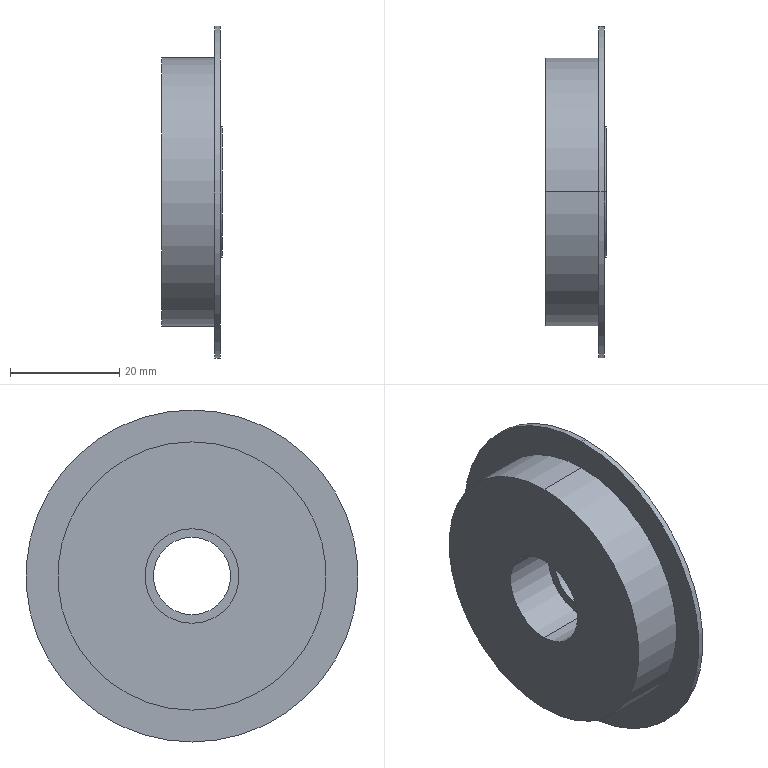Part | SolidWorks | features Revolution 1 | 2 solids | 18 faces | box 11.085 x 60.752 x 60.752 mm | volume 17812 mm3 | cylinder 12 | plane 6 | commonest cylinder face diameters 14.183 x2 17.319 x2 23.998 x2 45.246 x2 49.1 x2 60.752 x2
STEP:
#1=CARTESIAN_POINT('',(108.,0.,22.623));
#2=VERTEX_POINT('',#1);
#3=CARTESIAN_POINT('',(108.,0.,-22.623));
#4=VERTEX_POINT('',#3);
#5=CARTESIAN_POINT('',(108.,0.,0.));
#6=DIRECTION('',(1.,0.,0.));
#7=DIRECTION('',(0.,0.,-1.));
#8=AXIS2_PLACEMENT_3D('',#5,#6,#7);
#9=CIRCLE('',#8,22.623);
#10=EDGE_CURVE('',#2,#4,#9,.T.);
#11=ORIENTED_EDGE('',*,*,#10,.F.);
#12=CARTESIAN_POINT('',(109.025,0.,22.623));
#13=VERTEX_POINT('',#12);
#14=CARTESIAN_POINT('',(0.,0.,22.623));
#15=DIRECTION('',(1.,0.,0.));
#16=VECTOR('',#15,1000.);
#17=LINE('',#14,#16);
#18=EDGE_CURVE('',#2,#13,#17,.T.);
#19=ORIENTED_EDGE('',*,*,#18,.T.);
#20=CARTESIAN_POINT('',(109.025,0.,-22.623));
#21=VERTEX_POINT('',#20);
#22=CARTESIAN_POINT('',(109.025,0.,0.));
#23=DIRECTION('',(1.,0.,0.));
#24=DIRECTION('',(0.,0.,-1.));
#25=AXIS2_PLACEMENT_3D('',#22,#23,#24);
#26=CIRCLE('',#25,22.623);
#27=EDGE_CURVE('',#13,#21,#26,.T.);
#28=ORIENTED_EDGE('',*,*,#27,.T.);
#29=CARTESIAN_POINT('',(0.,0.,-22.623));
#30=DIRECTION('',(1.,0.,0.));
#31=VECTOR('',#30,1000.);
#32=LINE('',#29,#31);
#33=EDGE_CURVE('',#4,#21,#32,.T.);
#34=ORIENTED_EDGE('',*,*,#33,.F.);
#35=EDGE_LOOP('',(#11,#19,#28,#34));
#36=FACE_OUTER_BOUND('',#35,.T.);
#37=CARTESIAN_POINT('',(0.,0.,0.));
#38=DIRECTION('',(1.,0.,0.));
#39=DIRECTION('',(0.,0.,-1.));
#40=AXIS2_PLACEMENT_3D('',#37,#38,#39);
#41=CYLINDRICAL_SURFACE('',#40,22.623);
#42=ADVANCED_FACE('',(#36),#41,.F.);
#43=CARTESIAN_POINT('',(98.286,0.,8.66));
#44=VERTEX_POINT('',#43);
#45=CARTESIAN_POINT('',(98.286,0.,-8.66));
#46=VERTEX_POINT('',#45);
#47=CARTESIAN_POINT('',(98.286,0.,0.));
#48=DIRECTION('',(1.,0.,0.));
#49=DIRECTION('',(0.,0.,-1.));
#50=AXIS2_PLACEMENT_3D('',#47,#48,#49);
#51=CIRCLE('',#50,8.66);
#52=EDGE_CURVE('',#44,#46,#51,.T.);
#53=ORIENTED_EDGE('',*,*,#52,.F.);
#54=CARTESIAN_POINT('',(108.,0.,8.66));
#55=VERTEX_POINT('',#54);
#56=CARTESIAN_POINT('',(0.,0.,8.66));
#57=DIRECTION('',(1.,0.,0.));
#58=VECTOR('',#57,1000.);
#59=LINE('',#56,#58);
#60=EDGE_CURVE('',#44,#55,#59,.T.);
#61=ORIENTED_EDGE('',*,*,#60,.T.);
#62=CARTESIAN_POINT('',(108.,0.,-8.66));
#63=VERTEX_POINT('',#62);
#64=CARTESIAN_POINT('',(108.,0.,0.));
#65=DIRECTION('',(1.,0.,0.));
#66=DIRECTION('',(0.,0.,-1.));
#67=AXIS2_PLACEMENT_3D('',#64,#65,#66);
#68=CIRCLE('',#67,8.66);
#69=EDGE_CURVE('',#55,#63,#68,.T.);
#70=ORIENTED_EDGE('',*,*,#69,.T.);
#71=CARTESIAN_POINT('',(0.,0.,-8.66));
#72=DIRECTION('',(1.,0.,0.));
#73=VECTOR('',#72,1000.);
#74=LINE('',#71,#73);
#75=EDGE_CURVE('',#46,#63,#74,.T.);
#76=ORIENTED_EDGE('',*,*,#75,.F.);
#77=EDGE_LOOP('',(#53,#61,#70,#76));
#78=FACE_OUTER_BOUND('',#77,.T.);
#79=CARTESIAN_POINT('',(0.,0.,0.));
#80=DIRECTION('',(1.,0.,0.));
#81=DIRECTION('',(0.,0.,-1.));
#82=AXIS2_PLACEMENT_3D('',#79,#80,#81);
#83=CYLINDRICAL_SURFACE('',#82,8.66);
#84=ADVANCED_FACE('',(#78),#83,.F.);
#85=CARTESIAN_POINT('',(98.286,0.,-24.55));
#86=VERTEX_POINT('',#85);
#87=CARTESIAN_POINT('',(98.286,0.,24.55));
#88=VERTEX_POINT('',#87);
#89=CARTESIAN_POINT('',(98.286,0.,0.));
#90=DIRECTION('',(1.,0.,0.));
#91=DIRECTION('',(0.,0.,-1.));
#92=AXIS2_PLACEMENT_3D('',#89,#90,#91);
#93=CIRCLE('',#92,24.55);
#94=EDGE_CURVE('',#86,#88,#93,.T.);
#95=ORIENTED_EDGE('',*,*,#94,.T.);
#96=CARTESIAN_POINT('',(108.,0.,24.55));
#97=VERTEX_POINT('',#96);
#98=CARTESIAN_POINT('',(0.,0.,24.55));
#99=DIRECTION('',(1.,0.,0.));
#100=VECTOR('',#99,1000.);
#101=LINE('',#98,#100);
#102=EDGE_CURVE('',#88,#97,#101,.T.);
#103=ORIENTED_EDGE('',*,*,#102,.T.);
#104=CARTESIAN_POINT('',(108.,0.,-24.55));
#105=VERTEX_POINT('',#104);
#106=CARTESIAN_POINT('',(108.,0.,0.));
#107=DIRECTION('',(1.,0.,0.));
#108=DIRECTION('',(0.,0.,-1.));
#109=AXIS2_PLACEMENT_3D('',#106,#107,#108);
#110=CIRCLE('',#109,24.55);
#111=EDGE_CURVE('',#105,#97,#110,.T.);
#112=ORIENTED_EDGE('',*,*,#111,.F.);
#113=CARTESIAN_POINT('',(0.,0.,-24.55));
#114=DIRECTION('',(1.,0.,0.));
#115=VECTOR('',#114,1000.);
#116=LINE('',#113,#115);
#117=EDGE_CURVE('',#86,#105,#116,.T.);
#118=ORIENTED_EDGE('',*,*,#117,.F.);
#119=EDGE_LOOP('',(#95,#103,#112,#118));
#120=FACE_OUTER_BOUND('',#119,.T.);
#121=CARTESIAN_POINT('',(0.,0.,0.));
#122=DIRECTION('',(1.,0.,0.));
#123=DIRECTION('',(0.,0.,-1.));
#124=AXIS2_PLACEMENT_3D('',#121,#122,#123);
#125=CYLINDRICAL_SURFACE('',#124,24.55);
#126=ADVANCED_FACE('',(#120),#125,.T.);
#127=CARTESIAN_POINT('',(108.,0.,-30.376));
#128=VERTEX_POINT('',#127);
#129=CARTESIAN_POINT('',(108.,0.,30.376));
#130=VERTEX_POINT('',#129);
#131=CARTESIAN_POINT('',(108.,0.,0.));
#132=DIRECTION('',(1.,0.,0.));
#133=DIRECTION('',(0.,0.,-1.));
#134=AXIS2_PLACEMENT_3D('',#131,#132,#133);
#135=CIRCLE('',#134,30.376);
#136=EDGE_CURVE('',#128,#130,#135,.T.);
#137=ORIENTED_EDGE('',*,*,#136,.T.);
#138=CARTESIAN_POINT('',(109.025,0.,30.376));
#139=VERTEX_POINT('',#138);
#140=CARTESIAN_POINT('',(0.,0.,30.376));
#141=DIRECTION('',(1.,0.,0.));
#142=VECTOR('',#141,1000.);
#143=LINE('',#140,#142);
#144=EDGE_CURVE('',#130,#139,#143,.T.);
#145=ORIENTED_EDGE('',*,*,#144,.T.);
#146=CARTESIAN_POINT('',(109.025,0.,-30.376));
#147=VERTEX_POINT('',#146);
#148=CARTESIAN_POINT('',(109.025,0.,0.));
#149=DIRECTION('',(1.,0.,0.));
#150=DIRECTION('',(0.,0.,-1.));
#151=AXIS2_PLACEMENT_3D('',#148,#149,#150);
#152=CIRCLE('',#151,30.376);
#153=EDGE_CURVE('',#147,#139,#152,.T.);
#154=ORIENTED_EDGE('',*,*,#153,.F.);
#155=CARTESIAN_POINT('',(0.,0.,-30.376));
#156=DIRECTION('',(1.,0.,0.));
#157=VECTOR('',#156,1000.);
#158=LINE('',#155,#157);
#159=EDGE_CURVE('',#128,#147,#158,.T.);
#160=ORIENTED_EDGE('',*,*,#159,.F.);
#161=EDGE_LOOP('',(#137,#145,#154,#160));
#162=FACE_OUTER_BOUND('',#161,.T.);
#163=CARTESIAN_POINT('',(0.,0.,0.));
#164=DIRECTION('',(1.,0.,0.));
#165=DIRECTION('',(0.,0.,-1.));
#166=AXIS2_PLACEMENT_3D('',#163,#164,#165);
#167=CYLINDRICAL_SURFACE('',#166,30.376);
#168=ADVANCED_FACE('',(#162),#167,.T.);
#169=ORIENTED_EDGE('',*,*,#144,.F.);
#170=CARTESIAN_POINT('',(108.,0.,0.));
#171=DIRECTION('',(1.,0.,0.));
#172=DIRECTION('',(0.,0.,-1.));
#173=AXIS2_PLACEMENT_3D('',#170,#171,#172);
#174=CIRCLE('',#173,30.376);
#175=EDGE_CURVE('',#130,#128,#174,.T.);
#176=ORIENTED_EDGE('',*,*,#175,.T.);
#177=ORIENTED_EDGE('',*,*,#159,.T.);
#178=CARTESIAN_POINT('',(109.025,0.,0.));
#179=DIRECTION('',(1.,0.,0.));
#180=DIRECTION('',(0.,0.,-1.));
#181=AXIS2_PLACEMENT_3D('',#178,#179,#180);
#182=CIRCLE('',#181,30.376);
#183=EDGE_CURVE('',#139,#147,#182,.T.);
#184=ORIENTED_EDGE('',*,*,#183,.F.);
#185=EDGE_LOOP('',(#169,#176,#177,#184));
#186=FACE_OUTER_BOUND('',#185,.T.);
#187=CARTESIAN_POINT('',(0.,0.,0.));
#188=DIRECTION('',(1.,0.,0.));
#189=DIRECTION('',(0.,0.,-1.));
#190=AXIS2_PLACEMENT_3D('',#187,#188,#189);
#191=CYLINDRICAL_SURFACE('',#190,30.376);
#192=ADVANCED_FACE('',(#186),#191,.T.);
#193=ORIENTED_EDGE('',*,*,#111,.T.);
#194=CARTESIAN_POINT('',(108.,0.,0.));
#195=DIRECTION('',(1.,0.,0.));
#196=DIRECTION('',(0.,0.,-1.));
#197=AXIS2_PLACEMENT_3D('',#194,#195,#196);
#198=CIRCLE('',#197,24.55);
#199=EDGE_CURVE('',#97,#105,#198,.T.);
#200=ORIENTED_EDGE('',*,*,#199,.T.);
#201=EDGE_LOOP('',(#193,#200));
#202=FACE_BOUND('',#201,.T.);
#203=ORIENTED_EDGE('',*,*,#136,.F.);
#204=ORIENTED_EDGE('',*,*,#175,.F.);
#205=EDGE_LOOP('',(#203,#204));
#206=FACE_OUTER_BOUND('',#205,.T.);
#207=CARTESIAN_POINT('',(108.,30.376,0.));
#208=DIRECTION('',(-1.,0.,0.));
#209=DIRECTION('',(0.,0.,1.));
#210=AXIS2_PLACEMENT_3D('',#207,#208,#209);
#211=PLANE('',#210);
#212=ADVANCED_FACE('',(#202,#206),#211,.T.);
#213=ORIENTED_EDGE('',*,*,#102,.F.);
#214=CARTESIAN_POINT('',(98.286,0.,0.));
#215=DIRECTION('',(1.,0.,0.));
#216=DIRECTION('',(0.,0.,-1.));
#217=AXIS2_PLACEMENT_3D('',#214,#215,#216);
#218=CIRCLE('',#217,24.55);
#219=EDGE_CURVE('',#88,#86,#218,.T.);
#220=ORIENTED_EDGE('',*,*,#219,.T.);
#221=ORIENTED_EDGE('',*,*,#117,.T.);
#222=ORIENTED_EDGE('',*,*,#199,.F.);
#223=EDGE_LOOP('',(#213,#220,#221,#222));
#224=FACE_OUTER_BOUND('',#223,.T.);
#225=CARTESIAN_POINT('',(0.,0.,0.));
#226=DIRECTION('',(1.,0.,0.));
#227=DIRECTION('',(0.,0.,-1.));
#228=AXIS2_PLACEMENT_3D('',#225,#226,#227);
#229=CYLINDRICAL_SURFACE('',#228,24.55);
#230=ADVANCED_FACE('',(#224),#229,.T.);
#231=CARTESIAN_POINT('',(98.286,0.,0.));
#232=DIRECTION('',(1.,0.,0.));
#233=DIRECTION('',(0.,0.,-1.));
#234=AXIS2_PLACEMENT_3D('',#231,#232,#233);
#235=CIRCLE('',#234,8.66);
#236=EDGE_CURVE('',#46,#44,#235,.T.);
#237=ORIENTED_EDGE('',*,*,#236,.T.);
#238=ORIENTED_EDGE('',*,*,#52,.T.);
#239=EDGE_LOOP('',(#237,#238));
#240=FACE_BOUND('',#239,.T.);
#241=ORIENTED_EDGE('',*,*,#94,.F.);
#242=ORIENTED_EDGE('',*,*,#219,.F.);
#243=EDGE_LOOP('',(#241,#242));
#244=FACE_OUTER_BOUND('',#243,.T.);
#245=CARTESIAN_POINT('',(98.286,24.55,0.));
#246=DIRECTION('',(-1.,0.,0.));
#247=DIRECTION('',(0.,0.,1.));
#248=AXIS2_PLACEMENT_3D('',#245,#246,#247);
#249=PLANE('',#248);
#250=ADVANCED_FACE('',(#240,#244),#249,.T.);
#251=ORIENTED_EDGE('',*,*,#60,.F.);
#252=ORIENTED_EDGE('',*,*,#236,.F.);
#253=ORIENTED_EDGE('',*,*,#75,.T.);
#254=CARTESIAN_POINT('',(108.,0.,0.));
#255=DIRECTION('',(1.,0.,0.));
#256=DIRECTION('',(0.,0.,-1.));
#257=AXIS2_PLACEMENT_3D('',#254,#255,#256);
#258=CIRCLE('',#257,8.66);
#259=EDGE_CURVE('',#63,#55,#258,.T.);
#260=ORIENTED_EDGE('',*,*,#259,.T.);
#261=EDGE_LOOP('',(#251,#252,#253,#260));
#262=FACE_OUTER_BOUND('',#261,.T.);
#263=CARTESIAN_POINT('',(0.,0.,0.));
#264=DIRECTION('',(1.,0.,0.));
#265=DIRECTION('',(0.,0.,-1.));
#266=AXIS2_PLACEMENT_3D('',#263,#264,#265);
#267=CYLINDRICAL_SURFACE('',#266,8.66);
#268=ADVANCED_FACE('',(#262),#267,.F.);
#269=CARTESIAN_POINT('',(108.,0.,0.));
#270=DIRECTION('',(1.,0.,0.));
#271=DIRECTION('',(0.,0.,-1.));
#272=AXIS2_PLACEMENT_3D('',#269,#270,#271);
#273=CIRCLE('',#272,22.623);
#274=EDGE_CURVE('',#4,#2,#273,.T.);
#275=ORIENTED_EDGE('',*,*,#274,.T.);
#276=ORIENTED_EDGE('',*,*,#10,.T.);
#277=EDGE_LOOP('',(#275,#276));
#278=FACE_OUTER_BOUND('',#277,.T.);
#279=ORIENTED_EDGE('',*,*,#259,.F.);
#280=ORIENTED_EDGE('',*,*,#69,.F.);
#281=EDGE_LOOP('',(#279,#280));
#282=FACE_BOUND('',#281,.T.);
#283=CARTESIAN_POINT('',(108.,8.66,0.));
#284=DIRECTION('',(1.,0.,0.));
#285=DIRECTION('',(0.,0.,-1.));
#286=AXIS2_PLACEMENT_3D('',#283,#284,#285);
#287=PLANE('',#286);
#288=ADVANCED_FACE('',(#278,#282),#287,.T.);
#289=ORIENTED_EDGE('',*,*,#18,.F.);
#290=ORIENTED_EDGE('',*,*,#274,.F.);
#291=ORIENTED_EDGE('',*,*,#33,.T.);
#292=CARTESIAN_POINT('',(109.025,0.,0.));
#293=DIRECTION('',(1.,0.,0.));
#294=DIRECTION('',(0.,0.,-1.));
#295=AXIS2_PLACEMENT_3D('',#292,#293,#294);
#296=CIRCLE('',#295,22.623);
#297=EDGE_CURVE('',#21,#13,#296,.T.);
#298=ORIENTED_EDGE('',*,*,#297,.T.);
#299=EDGE_LOOP('',(#289,#290,#291,#298));
#300=FACE_OUTER_BOUND('',#299,.T.);
#301=CARTESIAN_POINT('',(0.,0.,0.));
#302=DIRECTION('',(1.,0.,0.));
#303=DIRECTION('',(0.,0.,-1.));
#304=AXIS2_PLACEMENT_3D('',#301,#302,#303);
#305=CYLINDRICAL_SURFACE('',#304,22.623);
#306=ADVANCED_FACE('',(#300),#305,.F.);
#307=ORIENTED_EDGE('',*,*,#153,.T.);
#308=ORIENTED_EDGE('',*,*,#183,.T.);
#309=EDGE_LOOP('',(#307,#308));
#310=FACE_OUTER_BOUND('',#309,.T.);
#311=ORIENTED_EDGE('',*,*,#297,.F.);
#312=ORIENTED_EDGE('',*,*,#27,.F.);
#313=EDGE_LOOP('',(#311,#312));
#314=FACE_BOUND('',#313,.T.);
#315=CARTESIAN_POINT('',(109.025,22.623,0.));
#316=DIRECTION('',(1.,0.,0.));
#317=DIRECTION('',(0.,0.,-1.));
#318=AXIS2_PLACEMENT_3D('',#315,#316,#317);
#319=PLANE('',#318);
#320=ADVANCED_FACE('',(#310,#314),#319,.T.);
#321=CLOSED_SHELL('',(#42,#84,#126,#168,#192,#212,#230,#250,#268,#288,#306,#320));
#322=MANIFOLD_SOLID_BREP('',#321);
#323=CARTESIAN_POINT('',(108.065,0.,7.092));
#324=VERTEX_POINT('',#323);
#325=CARTESIAN_POINT('',(108.065,0.,-7.092));
#326=VERTEX_POINT('',#325);
#327=CARTESIAN_POINT('',(108.065,0.,0.));
#328=DIRECTION('',(1.,0.,0.));
#329=DIRECTION('',(0.,0.,-1.));
#330=AXIS2_PLACEMENT_3D('',#327,#328,#329);
#331=CIRCLE('',#330,7.092);
#332=EDGE_CURVE('',#324,#326,#331,.T.);
#333=ORIENTED_EDGE('',*,*,#332,.F.);
#334=CARTESIAN_POINT('',(109.372,0.,7.092));
#335=VERTEX_POINT('',#334);
#336=CARTESIAN_POINT('',(0.,0.,7.092));
#337=DIRECTION('',(1.,0.,0.));
#338=VECTOR('',#337,1000.);
#339=LINE('',#336,#338);
#340=EDGE_CURVE('',#324,#335,#339,.T.);
#341=ORIENTED_EDGE('',*,*,#340,.T.);
#342=CARTESIAN_POINT('',(109.372,0.,-7.092));
#343=VERTEX_POINT('',#342);
#344=CARTESIAN_POINT('',(109.372,0.,0.));
#345=DIRECTION('',(1.,0.,0.));
#346=DIRECTION('',(0.,0.,-1.));
#347=AXIS2_PLACEMENT_3D('',#344,#345,#346);
#348=CIRCLE('',#347,7.092);
#349=EDGE_CURVE('',#335,#343,#348,.T.);
#350=ORIENTED_EDGE('',*,*,#349,.T.);
#351=CARTESIAN_POINT('',(0.,0.,-7.092));
#352=DIRECTION('',(1.,0.,0.));
#353=VECTOR('',#352,1000.);
#354=LINE('',#351,#353);
#355=EDGE_CURVE('',#326,#343,#354,.T.);
#356=ORIENTED_EDGE('',*,*,#355,.F.);
#357=EDGE_LOOP('',(#333,#341,#350,#356));
#358=FACE_OUTER_BOUND('',#357,.T.);
#359=CARTESIAN_POINT('',(0.,0.,0.));
#360=DIRECTION('',(1.,0.,0.));
#361=DIRECTION('',(0.,0.,-1.));
#362=AXIS2_PLACEMENT_3D('',#359,#360,#361);
#363=CYLINDRICAL_SURFACE('',#362,7.092);
#364=ADVANCED_FACE('',(#358),#363,.F.);
#365=CARTESIAN_POINT('',(108.065,0.,-11.999));
#366=VERTEX_POINT('',#365);
#367=CARTESIAN_POINT('',(108.065,0.,11.999));
#368=VERTEX_POINT('',#367);
#369=CARTESIAN_POINT('',(108.065,0.,0.));
#370=DIRECTION('',(1.,0.,0.));
#371=DIRECTION('',(0.,0.,-1.));
#372=AXIS2_PLACEMENT_3D('',#369,#370,#371);
#373=CIRCLE('',#372,11.999);
#374=EDGE_CURVE('',#366,#368,#373,.T.);
#375=ORIENTED_EDGE('',*,*,#374,.T.);
#376=CARTESIAN_POINT('',(109.372,0.,11.999));
#377=VERTEX_POINT('',#376);
#378=CARTESIAN_POINT('',(0.,0.,11.999));
#379=DIRECTION('',(1.,0.,0.));
#380=VECTOR('',#379,1000.);
#381=LINE('',#378,#380);
#382=EDGE_CURVE('',#368,#377,#381,.T.);
#383=ORIENTED_EDGE('',*,*,#382,.T.);
#384=CARTESIAN_POINT('',(109.372,0.,-11.999));
#385=VERTEX_POINT('',#384);
#386=CARTESIAN_POINT('',(109.372,0.,0.));
#387=DIRECTION('',(1.,0.,0.));
#388=DIRECTION('',(0.,0.,-1.));
#389=AXIS2_PLACEMENT_3D('',#386,#387,#388);
#390=CIRCLE('',#389,11.999);
#391=EDGE_CURVE('',#385,#377,#390,.T.);
#392=ORIENTED_EDGE('',*,*,#391,.F.);
#393=CARTESIAN_POINT('',(0.,0.,-11.999));
#394=DIRECTION('',(1.,0.,0.));
#395=VECTOR('',#394,1000.);
#396=LINE('',#393,#395);
#397=EDGE_CURVE('',#366,#385,#396,.T.);
#398=ORIENTED_EDGE('',*,*,#397,.F.);
#399=EDGE_LOOP('',(#375,#383,#392,#398));
#400=FACE_OUTER_BOUND('',#399,.T.);
#401=CARTESIAN_POINT('',(0.,0.,0.));
#402=DIRECTION('',(1.,0.,0.));
#403=DIRECTION('',(0.,0.,-1.));
#404=AXIS2_PLACEMENT_3D('',#401,#402,#403);
#405=CYLINDRICAL_SURFACE('',#404,11.999);
#406=ADVANCED_FACE('',(#400),#405,.T.);
#407=CARTESIAN_POINT('',(108.065,0.,0.));
#408=DIRECTION('',(1.,0.,0.));
#409=DIRECTION('',(0.,0.,-1.));
#410=AXIS2_PLACEMENT_3D('',#407,#408,#409);
#411=CIRCLE('',#410,7.092);
#412=EDGE_CURVE('',#326,#324,#411,.T.);
#413=ORIENTED_EDGE('',*,*,#412,.T.);
#414=ORIENTED_EDGE('',*,*,#332,.T.);
#415=EDGE_LOOP('',(#413,#414));
#416=FACE_BOUND('',#415,.T.);
#417=ORIENTED_EDGE('',*,*,#374,.F.);
#418=CARTESIAN_POINT('',(108.065,0.,0.));
#419=DIRECTION('',(1.,0.,0.));
#420=DIRECTION('',(0.,0.,-1.));
#421=AXIS2_PLACEMENT_3D('',#418,#419,#420);
#422=CIRCLE('',#421,11.999);
#423=EDGE_CURVE('',#368,#366,#422,.T.);
#424=ORIENTED_EDGE('',*,*,#423,.F.);
#425=EDGE_LOOP('',(#417,#424));
#426=FACE_OUTER_BOUND('',#425,.T.);
#427=CARTESIAN_POINT('',(108.065,7.092,0.));
#428=DIRECTION('',(-1.,0.,0.));
#429=DIRECTION('',(0.,0.,1.));
#430=AXIS2_PLACEMENT_3D('',#427,#428,#429);
#431=PLANE('',#430);
#432=ADVANCED_FACE('',(#416,#426),#431,.T.);
#433=ORIENTED_EDGE('',*,*,#382,.F.);
#434=ORIENTED_EDGE('',*,*,#423,.T.);
#435=ORIENTED_EDGE('',*,*,#397,.T.);
#436=CARTESIAN_POINT('',(109.372,0.,0.));
#437=DIRECTION('',(1.,0.,0.));
#438=DIRECTION('',(0.,0.,-1.));
#439=AXIS2_PLACEMENT_3D('',#436,#437,#438);
#440=CIRCLE('',#439,11.999);
#441=EDGE_CURVE('',#377,#385,#440,.T.);
#442=ORIENTED_EDGE('',*,*,#441,.F.);
#443=EDGE_LOOP('',(#433,#434,#435,#442));
#444=FACE_OUTER_BOUND('',#443,.T.);
#445=CARTESIAN_POINT('',(0.,0.,0.));
#446=DIRECTION('',(1.,0.,0.));
#447=DIRECTION('',(0.,0.,-1.));
#448=AXIS2_PLACEMENT_3D('',#445,#446,#447);
#449=CYLINDRICAL_SURFACE('',#448,11.999);
#450=ADVANCED_FACE('',(#444),#449,.T.);
#451=ORIENTED_EDGE('',*,*,#391,.T.);
#452=ORIENTED_EDGE('',*,*,#441,.T.);
#453=EDGE_LOOP('',(#451,#452));
#454=FACE_OUTER_BOUND('',#453,.T.);
#455=CARTESIAN_POINT('',(109.372,0.,0.));
#456=DIRECTION('',(1.,0.,0.));
#457=DIRECTION('',(0.,0.,-1.));
#458=AXIS2_PLACEMENT_3D('',#455,#456,#457);
#459=CIRCLE('',#458,7.092);
#460=EDGE_CURVE('',#343,#335,#459,.T.);
#461=ORIENTED_EDGE('',*,*,#460,.F.);
#462=ORIENTED_EDGE('',*,*,#349,.F.);
#463=EDGE_LOOP('',(#461,#462));
#464=FACE_BOUND('',#463,.T.);
#465=CARTESIAN_POINT('',(109.372,7.092,0.));
#466=DIRECTION('',(1.,0.,0.));
#467=DIRECTION('',(0.,0.,-1.));
#468=AXIS2_PLACEMENT_3D('',#465,#466,#467);
#469=PLANE('',#468);
#470=ADVANCED_FACE('',(#454,#464),#469,.T.);
#471=ORIENTED_EDGE('',*,*,#340,.F.);
#472=ORIENTED_EDGE('',*,*,#412,.F.);
#473=ORIENTED_EDGE('',*,*,#355,.T.);
#474=ORIENTED_EDGE('',*,*,#460,.T.);
#475=EDGE_LOOP('',(#471,#472,#473,#474));
#476=FACE_OUTER_BOUND('',#475,.T.);
#477=CARTESIAN_POINT('',(0.,0.,0.));
#478=DIRECTION('',(1.,0.,0.));
#479=DIRECTION('',(0.,0.,-1.));
#480=AXIS2_PLACEMENT_3D('',#477,#478,#479);
#481=CYLINDRICAL_SURFACE('',#480,7.092);
#482=ADVANCED_FACE('',(#476),#481,.F.);
#483=CLOSED_SHELL('',(#364,#406,#432,#450,#470,#482));
#484=MANIFOLD_SOLID_BREP('',#483);
#485=CARTESIAN_POINT('',(0.,0.,0.));
#486=DIRECTION('',(0.,0.,1.));
#487=DIRECTION('',(1.,0.,0.));
#488=AXIS2_PLACEMENT_3D('',#485,#486,#487);
#489=(LENGTH_UNIT()NAMED_UNIT(*)SI_UNIT(.MILLI.,.METRE.));
#490=UNCERTAINTY_MEASURE_WITH_UNIT(LENGTH_MEASURE(0.00001),#489,'','');
#491=(NAMED_UNIT(*)PLANE_ANGLE_UNIT()SI_UNIT($,.RADIAN.));
#492=(NAMED_UNIT(*)SI_UNIT($,.STERADIAN.)SOLID_ANGLE_UNIT());
#493=(GEOMETRIC_REPRESENTATION_CONTEXT(3)GLOBAL_UNCERTAINTY_ASSIGNED_CONTEXT((#490))GLOBAL_UNIT_ASSIGNED_CONTEXT((#489,#491,#492))REPRESENTATION_CONTEXT('',''));
#494=ADVANCED_BREP_SHAPE_REPRESENTATION('',(#322,#484,#488),#493);